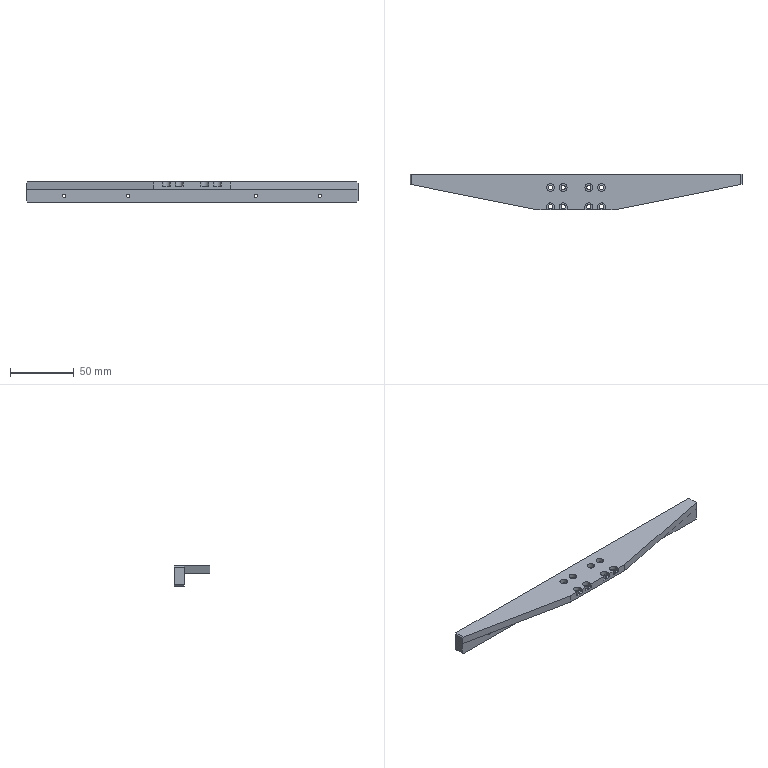NC program | NX | posted with a generic post | part box 260 x 28 x 16 mm
Whole program:
N10 G17 G21 G94 G90
(DRILLING_COPY_1 , TOOL : D6A45)
N12 T01 M6
N14 G54
N16 G17 G0 G90 X-120. Y-3. B0. C0. S9500 M3
N18 G43 Z30. H1
N20 G94 G81 G98 Z-1. F250. R3.
N22 X-112.5 Y0.
N24 X-100. Y3.
N26 X-60. Y-3.
N28 X-50. Y3.
N30 X0. Y-3.
N32 X50. Y3.
N34 X60. Y-3.
N36 X100. Y3.
N38 X112.5 Y0.
N40 X120. Y-3.
N42 G80
N44 G0 X120. Y-3. Z30.
N46 M5
(DRILLING_COPY_COPY , TOOL : 2.5ZT)
N48 T02 M6
N50 G54
N52 G17 G0 G90 X-120. Y-3. B0. C0. S2000 M3
N54 G43 Z30. H2
N56 G94 G83 G98 Z-8.251 F150. Q2. R3.
N58 X-100. Y3. Z-10.251
N60 X-60. Y-3. Z-8.251
N62 X-50. Y3. Z-10.251
N64 X0. Y-3. Z-8.251
N66 X50. Y3. Z-10.251
N68 X60. Y-3. Z-8.251
N70 X100. Y3. Z-10.251
N72 X120. Y-3. Z-8.251
N74 G80
N76 G0 X120. Y-3. Z30.
N78 M5
(HOLE_MILLING_1 , TOOL : D3)
N80 T03 M6
N82 G54
N84 G17 G0 G90 X-112.5 Y0. B0. C0. S9500 M3
N86 G43 Z30. H3
N88 Z0.5
N90 G94 G3 X-112.3 Y-0.2 R0.2 F1000.
N92 X-112.1 Y0. R0.2
N94 X-112.1 Y0. Z0.2 I-0.4 J0.
N96 X-112.1 Y0. Z-0.1 I-0.4 J0.
N98 X-112.1 Y0. Z-0.4 I-0.4 J0.
N100 X-112.1 Y0. Z-0.7 I-0.4 J0.
N102 X-112.1 Y0. Z-1. I-0.4 J0.
N104 X-112.1 Y0. Z-1.3 I-0.4 J0.
N106 X-112.1 Y0. Z-1.6 I-0.4 J0.
N108 X-112.1 Y0. Z-1.9 I-0.4 J0.
N110 X-112.1 Y0. Z-2.2 I-0.4 J0.
N112 X-112.1 Y0. Z-2.5 I-0.4 J0.
N114 X-112.1 Y0. Z-2.8 I-0.4 J0.
N116 X-112.1 Y0. Z-3.1 I-0.4 J0.
N118 X-112.1 Y0. Z-3.4 I-0.4 J0.
N120 X-112.1 Y0. Z-3.7 I-0.4 J0.
N122 X-112.1 Y0. Z-4. I-0.4 J0.
N124 X-112.1 Y0. Z-4.3 I-0.4 J0.
N126 X-112.1 Y0. Z-4.6 I-0.4 J0.
N128 X-112.1 Y0. Z-4.9 I-0.4 J0.
N130 X-112.1 Y0. Z-5.2 I-0.4 J0.
N132 X-112.1 Y0. Z-5.5 I-0.4 J0.
N134 X-112.1 Y0. Z-5.8 I-0.4 J0.
N136 X-112.7 Y-0.346 Z-6. R-0.4
N138 X-112.154 Y-0.2 R0.4
N140 X-112.7 Y-0.346 R-0.4
N142 X-112.427 Y-0.273 R0.2
N144 X-112.5 Y0. R0.2
N146 G0 Z30.
N148 X112.5
N150 Z0.5
N152 G3 X112.7 Y-0.2 R0.2
N154 X112.9 Y0. R0.2
N156 X112.9 Y0. Z0.2 I-0.4 J0.
N158 X112.9 Y0. Z-0.1 I-0.4 J0.
N160 X112.9 Y0. Z-0.4 I-0.4 J0.
N162 X112.9 Y0. Z-0.7 I-0.4 J0.
N164 X112.9 Y0. Z-1. I-0.4 J0.
N166 X112.9 Y0. Z-1.3 I-0.4 J0.
N168 X112.9 Y0. Z-1.6 I-0.4 J0.
N170 X112.9 Y0. Z-1.9 I-0.4 J0.
N172 X112.9 Y0. Z-2.2 I-0.4 J0.
N174 X112.9 Y0. Z-2.5 I-0.4 J0.
N176 X112.9 Y0. Z-2.8 I-0.4 J0.
N178 X112.9 Y0. Z-3.1 I-0.4 J0.
N180 X112.9 Y0. Z-3.4 I-0.4 J0.
N182 X112.9 Y0. Z-3.7 I-0.4 J0.
N184 X112.9 Y0. Z-4. I-0.4 J0.
N186 X112.9 Y0. Z-4.3 I-0.4 J0.
N188 X112.9 Y0. Z-4.6 I-0.4 J0.
N190 X112.9 Y0. Z-4.9 I-0.4 J0.
N192 X112.9 Y0. Z-5.2 I-0.4 J0.
N194 X112.9 Y0. Z-5.5 I-0.4 J0.
N196 X112.9 Y0. Z-5.8 I-0.4 J0.
N198 X112.3 Y-0.346 Z-6. R-0.4
N200 X112.846 Y-0.2 R0.4
N202 X112.3 Y-0.346 R-0.4
N204 X112.573 Y-0.273 R0.2
N206 X112.5 Y0. R0.2
N208 G0 Z30.
N210 M5
(PLANAR_MILL_COPY_1_COPY , TOOL : D6A45)
N212 T01 M6
N214 G54
N216 G17 G0 G90 X120.217 Y-2.9 B0. C0. S9500 M3
N218 G43 Z30. H1
N220 Z0.5
N222 G94 G1 Z-1. F1250.
N224 G3 X120. Y-3.35 R0.5
N226 X120.35 Y-3. R0.35
N228 X120. Y-3.35 R-0.35
N230 X119.783 Y-2.9 R0.5
N232 G1 Z0.5
N234 G0 Z30.
N236 X111.634 Y-0.6
N238 Z0.5
N240 G1 Z-1.
N242 G3 X112.5 Y-1.1 R1.
N244 X113.6 Y0. R1.1
N246 X112.5 Y-1.1 R-1.1
N248 X113.366 Y-0.6 R1.
N250 G1 Z0.5
N252 G0 Z30.
N254 X99.783 Y2.9
N256 Z0.5
N258 G1 Z-1.
N260 G3 X100. Y3.35 R0.5
N262 X99.65 Y3. R0.35
N264 X100. Y3.35 R-0.35
N266 X100.217 Y2.9 R0.5
N268 G1 Z0.5
N270 G0 Z30.
N272 X60.217 Y-2.9
N274 Z0.5
N276 G1 Z-1.
N278 G3 X60. Y-3.35 R0.5
N280 X60.35 Y-3. R0.35
N282 X60. Y-3.35 R-0.35
N284 X59.783 Y-2.9 R0.5
N286 G1 Z0.5
N288 G0 Z30.
N290 X49.783 Y2.9
N292 Z0.5
N294 G1 Z-1.
N296 G3 X50. Y3.35 R0.5
N298 X49.65 Y3. R0.35
N300 X50. Y3.35 R-0.35
N302 X50.217 Y2.9 R0.5
N304 G1 Z0.5
N306 G0 Z30.
N308 X-0.866 Y9.4
N310 Z0.5
N312 G1 Z-1.
N314 G3 X0. Y8.9 R1.
N316 G1 X129.
N318 G2 X129.636 Y8.636 R0.9
N320 G1 X130.636 Y7.636
N322 G2 X130.9 Y7. R0.9
N324 G1 Y-7.
N326 G2 X130.636 Y-7.636 R0.9
N328 G1 X129.636 Y-8.636
N330 G2 X129. Y-8.9 R0.9
N332 G1 X-129.
N334 G2 X-129.636 Y-8.636 R0.9
N336 G1 X-130.636 Y-7.636
N338 G2 X-130.9 Y-7. R0.9
N340 G1 Y7.
N342 G2 X-130.636 Y7.636 R0.9
N344 G1 X-129.636 Y8.636
N346 G2 X-129. Y8.9 R0.9
N348 G1 X0.
N350 G3 X0.866 Y9.4 R1.
N352 G1 Z0.5
N354 G0 Z30.
N356 X0.217 Y-2.9
N358 Z0.5
N360 G1 Z-1.
N362 G3 X0. Y-3.35 R0.5
N364 X0.35 Y-3. R0.35
N366 X0. Y-3.35 R-0.35
N368 X-0.217 Y-2.9 R0.5
N370 G1 Z0.5
N372 G0 Z30.
N374 X-50.217 Y2.9
N376 Z0.5
N378 G1 Z-1.
N380 G3 X-50. Y3.35 R0.5
N382 X-50.35 Y3. R0.35
N384 X-50. Y3.35 R-0.35
N386 X-49.783 Y2.9 R0.5
N388 G1 Z0.5
N390 G0 Z30.
N392 X-59.783 Y-2.9
N394 Z0.5
N396 G1 Z-1.
N398 G3 X-60. Y-3.35 R0.5
N400 X-59.65 Y-3. R0.35
N402 X-60. Y-3.35 R-0.35
N404 X-60.217 Y-2.9 R0.5
N406 G1 Z0.5
N408 G0 Z30.
N410 X-100.217 Y2.9
N412 Z0.5
N414 G1 Z-1.
N416 G3 X-100. Y3.35 R0.5
N418 X-100.35 Y3. R0.35
N420 X-100. Y3.35 R-0.35
N422 X-99.783 Y2.9 R0.5
N424 G1 Z0.5
N426 G0 Z30.
N428 X-111.634 Y0.6
N430 Z0.5
N432 G1 Z-1.
N434 G3 X-112.5 Y1.1 R1.
N436 X-113.6 Y0. R1.1
N438 X-112.5 Y1.1 R-1.1
N440 X-113.366 Y0.6 R1.
N442 G1 Z0.5
N444 G0 Z30.
N446 X-119.783 Y-2.9
N448 Z0.5
N450 G1 Z-1.
N452 G3 X-120. Y-3.35 R0.5
N454 X-119.65 Y-3. R0.35
N456 X-120. Y-3.35 R-0.35
N458 X-120.217 Y-2.9 R0.5
N460 G1 Z0.5
N462 G0 Z30.
N464 M5
(刀补 , TOOL : D3)
N466 T03 M6
N468 G54
N470 G17 G0 G90 X-112.5 Y0. B0. C0. S9500 M3
N472 G43 Z30. H3
N474 Z0.5
N476 G41 G94 G1 X-112.473 Y-0.096 F1000. D3
N478 G3 X-112.05 Y0. R0.222
N480 X-112.05 Y0. Z-1.5 I-0.45 J0.
N482 X-112.05 Y0. Z-3.5 I-0.45 J0.
N484 X-112.05 Y0. Z-5.5 I-0.45 J0.
N486 X-112.5 Y0.45 Z-6. R0.45
N488 X-112.95 Y0. R0.45
N490 X-112.5 Y0.45 R-0.45
N492 X-112.596 Y0.027 R0.222
N494 G40
N496 G1 X-112.5 Y0.
N498 G0 Z30.
N500 X112.5
N502 Z0.5
N504 G41 G1 X112.527 Y-0.096
N506 G3 X112.95 Y0. R0.222
N508 X112.95 Y0. Z-1.5 I-0.45 J0.
N510 X112.95 Y0. Z-3.5 I-0.45 J0.
N512 X112.95 Y0. Z-5.5 I-0.45 J0.
N514 X112.5 Y0.45 Z-6. R0.45
N516 X112.05 Y0. R0.45
N518 X112.5 Y0.45 R-0.45
N520 X112.404 Y0.027 R0.222
N522 G40
N524 G1 X112.5 Y0.
N526 G0 Z30.
N528 M5
N530 M2